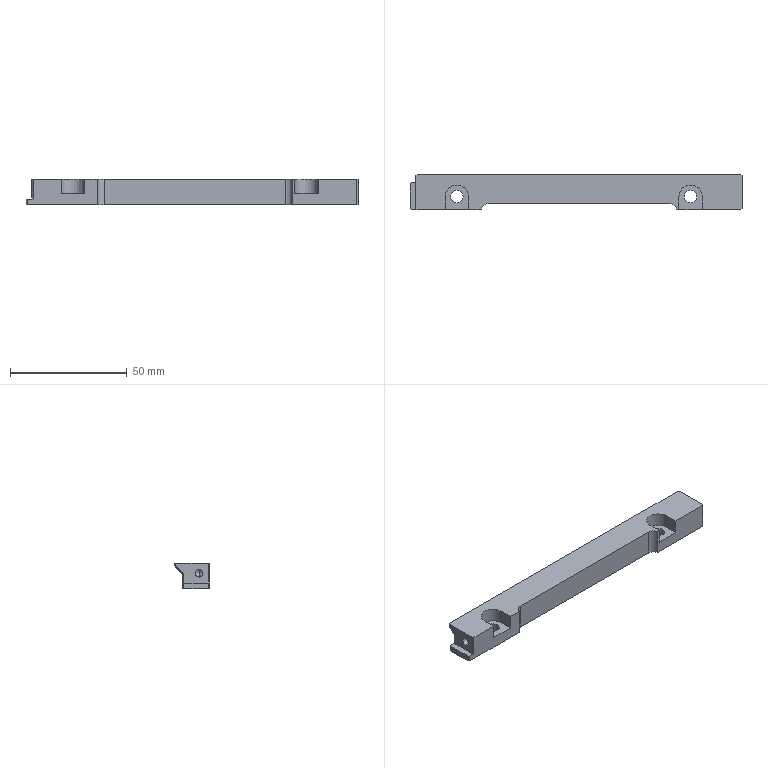Part | SolidWorks | features ICE 7, Chamfer 3, HoleWzd 2, Extrusion 1 | 1 solid | 51 faces | box 142 x 15 x 11 mm | volume 15061 mm3 | plane 32 | cylinder 17 | cone 2 | commonest cylinder face diameters 6 x7 5.4 x4 2.5 x2 3.3 x2 10 x2